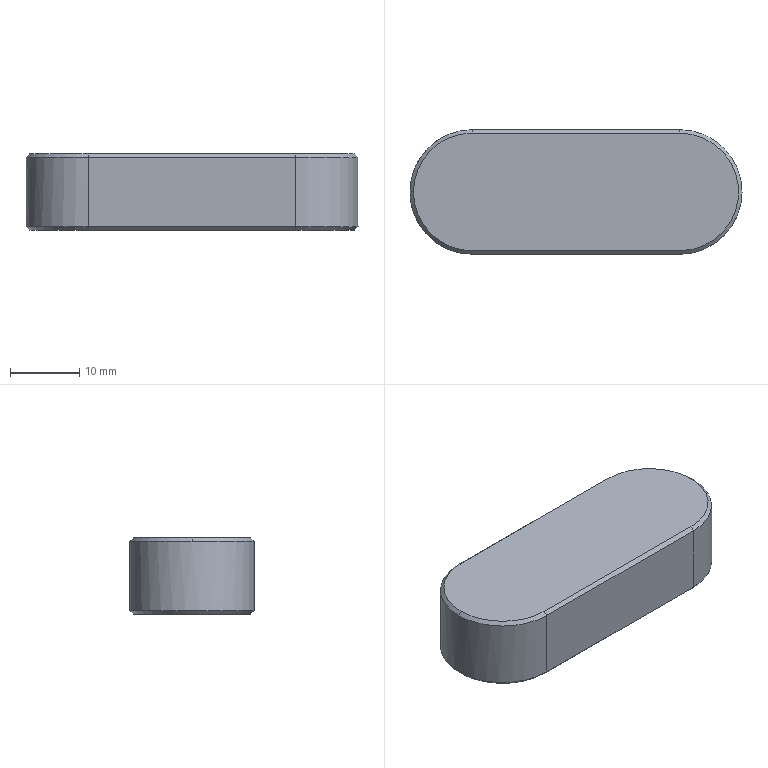Part | SolidWorks | features BaseBody 1 | 1 solid | 17 faces | box 48 x 18 x 11 mm | volume 8710 mm3 | plane 8 | cone 6 | cylinder 3 | commonest cylinder face diameters 18 x3
STEP:
#1=CARTESIAN_POINT('',(-18.723,2.01,11.));
#2=VERTEX_POINT('',#1);
#3=CARTESIAN_POINT('',(-10.223,-6.49,11.));
#4=VERTEX_POINT('',#3);
#5=CARTESIAN_POINT('',(-10.223,2.01,11.));
#6=DIRECTION('',(0.,0.,1.));
#7=DIRECTION('',(-1.,0.,0.));
#8=AXIS2_PLACEMENT_3D('',#5,#6,#7);
#9=CIRCLE('',#8,8.5);
#10=EDGE_CURVE('',#2,#4,#9,.T.);
#11=ORIENTED_EDGE('',*,*,#10,.F.);
#12=CARTESIAN_POINT('',(-19.223,2.01,10.5));
#13=VERTEX_POINT('',#12);
#14=CARTESIAN_POINT('',(-19.223,2.01,10.5));
#15=DIRECTION('',(-0.7071,0.,-0.7071));
#16=VECTOR('',#15,1000.);
#17=LINE('',#14,#16);
#18=EDGE_CURVE('',#2,#13,#17,.T.);
#19=ORIENTED_EDGE('',*,*,#18,.T.);
#20=CARTESIAN_POINT('',(-10.223,-6.99,10.5));
#21=VERTEX_POINT('',#20);
#22=CARTESIAN_POINT('',(-10.223,2.01,10.5));
#23=DIRECTION('',(0.,0.,1.));
#24=DIRECTION('',(0.,1.,0.));
#25=AXIS2_PLACEMENT_3D('',#22,#23,#24);
#26=CIRCLE('',#25,9.);
#27=EDGE_CURVE('',#13,#21,#26,.T.);
#28=ORIENTED_EDGE('',*,*,#27,.T.);
#29=CARTESIAN_POINT('',(-10.223,-6.74,10.75));
#30=DIRECTION('',(0.,0.7071,0.7071));
#31=VECTOR('',#30,1000.);
#32=LINE('',#29,#31);
#33=EDGE_CURVE('',#21,#4,#32,.T.);
#34=ORIENTED_EDGE('',*,*,#33,.T.);
#35=EDGE_LOOP('',(#11,#19,#28,#34));
#36=FACE_OUTER_BOUND('',#35,.T.);
#37=CARTESIAN_POINT('',(-10.223,2.01,10.5));
#38=DIRECTION('',(0.,0.,-1.));
#39=DIRECTION('',(-1.,0.,0.));
#40=AXIS2_PLACEMENT_3D('',#37,#38,#39);
#41=CONICAL_SURFACE('',#40,9.,0.7854);
#42=ADVANCED_FACE('',(#36),#41,.T.);
#43=CARTESIAN_POINT('',(19.777,-6.99,0.5));
#44=VERTEX_POINT('',#43);
#45=CARTESIAN_POINT('',(28.777,2.01,0.5));
#46=VERTEX_POINT('',#45);
#47=CARTESIAN_POINT('',(19.777,2.01,0.5));
#48=DIRECTION('',(0.,0.,1.));
#49=DIRECTION('',(1.,0.,0.));
#50=AXIS2_PLACEMENT_3D('',#47,#48,#49);
#51=CIRCLE('',#50,9.);
#52=EDGE_CURVE('',#44,#46,#51,.T.);
#53=ORIENTED_EDGE('',*,*,#52,.T.);
#54=CARTESIAN_POINT('',(28.777,2.01,10.5));
#55=VERTEX_POINT('',#54);
#56=CARTESIAN_POINT('',(28.777,2.01,0.));
#57=DIRECTION('',(0.,0.,1.));
#58=VECTOR('',#57,1000.);
#59=LINE('',#56,#58);
#60=EDGE_CURVE('',#46,#55,#59,.T.);
#61=ORIENTED_EDGE('',*,*,#60,.T.);
#62=CARTESIAN_POINT('',(19.777,-6.99,10.5));
#63=VERTEX_POINT('',#62);
#64=CARTESIAN_POINT('',(19.777,2.01,10.5));
#65=DIRECTION('',(0.,0.,1.));
#66=DIRECTION('',(0.,-1.,0.));
#67=AXIS2_PLACEMENT_3D('',#64,#65,#66);
#68=CIRCLE('',#67,9.);
#69=EDGE_CURVE('',#63,#55,#68,.T.);
#70=ORIENTED_EDGE('',*,*,#69,.F.);
#71=CARTESIAN_POINT('',(19.777,-6.99,0.));
#72=DIRECTION('',(0.,0.,-1.));
#73=VECTOR('',#72,1000.);
#74=LINE('',#71,#73);
#75=EDGE_CURVE('',#63,#44,#74,.T.);
#76=ORIENTED_EDGE('',*,*,#75,.T.);
#77=EDGE_LOOP('',(#53,#61,#70,#76));
#78=FACE_OUTER_BOUND('',#77,.T.);
#79=CARTESIAN_POINT('',(19.777,2.01,0.));
#80=DIRECTION('',(0.,0.,1.));
#81=DIRECTION('',(1.,0.,0.));
#82=AXIS2_PLACEMENT_3D('',#79,#80,#81);
#83=CYLINDRICAL_SURFACE('',#82,9.);
#84=ADVANCED_FACE('',(#78),#83,.T.);
#85=CARTESIAN_POINT('',(19.777,-6.49,0.));
#86=VERTEX_POINT('',#85);
#87=CARTESIAN_POINT('',(28.277,2.01,0.));
#88=VERTEX_POINT('',#87);
#89=CARTESIAN_POINT('',(19.777,2.01,0.));
#90=DIRECTION('',(0.,0.,1.));
#91=DIRECTION('',(1.,0.,0.));
#92=AXIS2_PLACEMENT_3D('',#89,#90,#91);
#93=CIRCLE('',#92,8.5);
#94=EDGE_CURVE('',#86,#88,#93,.T.);
#95=ORIENTED_EDGE('',*,*,#94,.T.);
#96=CARTESIAN_POINT('',(28.777,2.01,0.5));
#97=DIRECTION('',(0.7071,0.,0.7071));
#98=VECTOR('',#97,1000.);
#99=LINE('',#96,#98);
#100=EDGE_CURVE('',#88,#46,#99,.T.);
#101=ORIENTED_EDGE('',*,*,#100,.T.);
#102=ORIENTED_EDGE('',*,*,#52,.F.);
#103=CARTESIAN_POINT('',(19.777,-6.74,0.25));
#104=DIRECTION('',(0.,0.7071,-0.7071));
#105=VECTOR('',#104,1000.);
#106=LINE('',#103,#105);
#107=EDGE_CURVE('',#44,#86,#106,.T.);
#108=ORIENTED_EDGE('',*,*,#107,.T.);
#109=EDGE_LOOP('',(#95,#101,#102,#108));
#110=FACE_OUTER_BOUND('',#109,.T.);
#111=CARTESIAN_POINT('',(19.777,2.01,0.5));
#112=DIRECTION('',(0.,0.,1.));
#113=DIRECTION('',(1.,0.,0.));
#114=AXIS2_PLACEMENT_3D('',#111,#112,#113);
#115=CONICAL_SURFACE('',#114,9.,0.7854);
#116=ADVANCED_FACE('',(#110),#115,.T.);
#117=CARTESIAN_POINT('',(19.777,10.51,11.));
#118=VERTEX_POINT('',#117);
#119=CARTESIAN_POINT('',(-10.223,10.51,11.));
#120=VERTEX_POINT('',#119);
#121=CARTESIAN_POINT('',(4.777,10.51,11.));
#122=DIRECTION('',(-1.,0.,0.));
#123=VECTOR('',#122,1000.);
#124=LINE('',#121,#123);
#125=EDGE_CURVE('',#118,#120,#124,.T.);
#126=ORIENTED_EDGE('',*,*,#125,.T.);
#127=CARTESIAN_POINT('',(-10.223,2.01,11.));
#128=DIRECTION('',(0.,0.,1.));
#129=DIRECTION('',(-1.,0.,0.));
#130=AXIS2_PLACEMENT_3D('',#127,#128,#129);
#131=CIRCLE('',#130,8.5);
#132=EDGE_CURVE('',#120,#2,#131,.T.);
#133=ORIENTED_EDGE('',*,*,#132,.T.);
#134=ORIENTED_EDGE('',*,*,#10,.T.);
#135=CARTESIAN_POINT('',(19.777,-6.49,11.));
#136=VERTEX_POINT('',#135);
#137=CARTESIAN_POINT('',(4.777,-6.49,11.));
#138=DIRECTION('',(1.,0.,0.));
#139=VECTOR('',#138,1000.);
#140=LINE('',#137,#139);
#141=EDGE_CURVE('',#4,#136,#140,.T.);
#142=ORIENTED_EDGE('',*,*,#141,.T.);
#143=CARTESIAN_POINT('',(19.777,2.01,11.));
#144=DIRECTION('',(0.,0.,1.));
#145=DIRECTION('',(-1.,0.,0.));
#146=AXIS2_PLACEMENT_3D('',#143,#144,#145);
#147=CIRCLE('',#146,8.5);
#148=EDGE_CURVE('',#136,#118,#147,.T.);
#149=ORIENTED_EDGE('',*,*,#148,.T.);
#150=EDGE_LOOP('',(#126,#133,#134,#142,#149));
#151=FACE_OUTER_BOUND('',#150,.T.);
#152=CARTESIAN_POINT('',(4.777,2.01,11.));
#153=DIRECTION('',(0.,0.,1.));
#154=DIRECTION('',(1.,0.,0.));
#155=AXIS2_PLACEMENT_3D('',#152,#153,#154);
#156=PLANE('',#155);
#157=ADVANCED_FACE('',(#151),#156,.T.);
#158=ORIENTED_EDGE('',*,*,#18,.F.);
#159=ORIENTED_EDGE('',*,*,#132,.F.);
#160=CARTESIAN_POINT('',(-10.223,11.01,10.5));
#161=VERTEX_POINT('',#160);
#162=CARTESIAN_POINT('',(-10.223,10.76,10.75));
#163=DIRECTION('',(0.,0.7071,-0.7071));
#164=VECTOR('',#163,1000.);
#165=LINE('',#162,#164);
#166=EDGE_CURVE('',#120,#161,#165,.T.);
#167=ORIENTED_EDGE('',*,*,#166,.T.);
#168=CARTESIAN_POINT('',(-10.223,2.01,10.5));
#169=DIRECTION('',(0.,0.,1.));
#170=DIRECTION('',(0.,1.,0.));
#171=AXIS2_PLACEMENT_3D('',#168,#169,#170);
#172=CIRCLE('',#171,9.);
#173=EDGE_CURVE('',#161,#13,#172,.T.);
#174=ORIENTED_EDGE('',*,*,#173,.T.);
#175=EDGE_LOOP('',(#158,#159,#167,#174));
#176=FACE_OUTER_BOUND('',#175,.T.);
#177=CARTESIAN_POINT('',(-10.223,2.01,10.5));
#178=DIRECTION('',(0.,0.,-1.));
#179=DIRECTION('',(-1.,0.,0.));
#180=AXIS2_PLACEMENT_3D('',#177,#178,#179);
#181=CONICAL_SURFACE('',#180,9.,0.7854);
#182=ADVANCED_FACE('',(#176),#181,.T.);
#183=ORIENTED_EDGE('',*,*,#166,.F.);
#184=ORIENTED_EDGE('',*,*,#125,.F.);
#185=CARTESIAN_POINT('',(19.777,11.01,10.5));
#186=VERTEX_POINT('',#185);
#187=CARTESIAN_POINT('',(19.777,10.76,10.75));
#188=DIRECTION('',(0.,0.7071,-0.7071));
#189=VECTOR('',#188,1000.);
#190=LINE('',#187,#189);
#191=EDGE_CURVE('',#118,#186,#190,.T.);
#192=ORIENTED_EDGE('',*,*,#191,.T.);
#193=CARTESIAN_POINT('',(-2.723,11.01,10.5));
#194=DIRECTION('',(-1.,0.,0.));
#195=VECTOR('',#194,1000.);
#196=LINE('',#193,#195);
#197=EDGE_CURVE('',#186,#161,#196,.T.);
#198=ORIENTED_EDGE('',*,*,#197,.T.);
#199=EDGE_LOOP('',(#183,#184,#192,#198));
#200=FACE_OUTER_BOUND('',#199,.T.);
#201=CARTESIAN_POINT('',(-2.723,10.76,10.75));
#202=DIRECTION('',(0.,0.7071,0.7071));
#203=DIRECTION('',(0.,-0.7071,0.7071));
#204=AXIS2_PLACEMENT_3D('',#201,#202,#203);
#205=PLANE('',#204);
#206=ADVANCED_FACE('',(#200),#205,.T.);
#207=CARTESIAN_POINT('',(19.777,-6.74,10.75));
#208=DIRECTION('',(0.,-0.7071,-0.7071));
#209=VECTOR('',#208,1000.);
#210=LINE('',#207,#209);
#211=EDGE_CURVE('',#136,#63,#210,.T.);
#212=ORIENTED_EDGE('',*,*,#211,.T.);
#213=ORIENTED_EDGE('',*,*,#69,.T.);
#214=CARTESIAN_POINT('',(19.777,2.01,10.5));
#215=DIRECTION('',(0.,0.,1.));
#216=DIRECTION('',(0.,-1.,0.));
#217=AXIS2_PLACEMENT_3D('',#214,#215,#216);
#218=CIRCLE('',#217,9.);
#219=EDGE_CURVE('',#55,#186,#218,.T.);
#220=ORIENTED_EDGE('',*,*,#219,.T.);
#221=ORIENTED_EDGE('',*,*,#191,.F.);
#222=ORIENTED_EDGE('',*,*,#148,.F.);
#223=EDGE_LOOP('',(#212,#213,#220,#221,#222));
#224=FACE_OUTER_BOUND('',#223,.T.);
#225=CARTESIAN_POINT('',(19.777,2.01,10.5));
#226=DIRECTION('',(0.,0.,-1.));
#227=DIRECTION('',(-1.,0.,0.));
#228=AXIS2_PLACEMENT_3D('',#225,#226,#227);
#229=CONICAL_SURFACE('',#228,9.,0.7854);
#230=ADVANCED_FACE('',(#224),#229,.T.);
#231=ORIENTED_EDGE('',*,*,#33,.F.);
#232=CARTESIAN_POINT('',(12.277,-6.99,10.5));
#233=DIRECTION('',(1.,0.,0.));
#234=VECTOR('',#233,1000.);
#235=LINE('',#232,#234);
#236=EDGE_CURVE('',#21,#63,#235,.T.);
#237=ORIENTED_EDGE('',*,*,#236,.T.);
#238=ORIENTED_EDGE('',*,*,#211,.F.);
#239=ORIENTED_EDGE('',*,*,#141,.F.);
#240=EDGE_LOOP('',(#231,#237,#238,#239));
#241=FACE_OUTER_BOUND('',#240,.T.);
#242=CARTESIAN_POINT('',(12.277,-6.74,10.75));
#243=DIRECTION('',(0.,-0.7071,0.7071));
#244=DIRECTION('',(0.,-0.7071,-0.7071));
#245=AXIS2_PLACEMENT_3D('',#242,#243,#244);
#246=PLANE('',#245);
#247=ADVANCED_FACE('',(#241),#246,.T.);
#248=ORIENTED_EDGE('',*,*,#173,.F.);
#249=CARTESIAN_POINT('',(-10.223,11.01,0.5));
#250=VERTEX_POINT('',#249);
#251=CARTESIAN_POINT('',(-10.223,11.01,0.));
#252=DIRECTION('',(0.,0.,-1.));
#253=VECTOR('',#252,1000.);
#254=LINE('',#251,#253);
#255=EDGE_CURVE('',#161,#250,#254,.T.);
#256=ORIENTED_EDGE('',*,*,#255,.T.);
#257=CARTESIAN_POINT('',(-10.223,-6.99,0.5));
#258=VERTEX_POINT('',#257);
#259=CARTESIAN_POINT('',(-10.223,2.01,0.5));
#260=DIRECTION('',(0.,0.,1.));
#261=DIRECTION('',(1.,0.,0.));
#262=AXIS2_PLACEMENT_3D('',#259,#260,#261);
#263=CIRCLE('',#262,9.);
#264=EDGE_CURVE('',#250,#258,#263,.T.);
#265=ORIENTED_EDGE('',*,*,#264,.T.);
#266=CARTESIAN_POINT('',(-10.223,-6.99,0.));
#267=DIRECTION('',(0.,0.,1.));
#268=VECTOR('',#267,1000.);
#269=LINE('',#266,#268);
#270=EDGE_CURVE('',#258,#21,#269,.T.);
#271=ORIENTED_EDGE('',*,*,#270,.T.);
#272=ORIENTED_EDGE('',*,*,#27,.F.);
#273=EDGE_LOOP('',(#248,#256,#265,#271,#272));
#274=FACE_OUTER_BOUND('',#273,.T.);
#275=CARTESIAN_POINT('',(-10.223,2.01,0.));
#276=DIRECTION('',(0.,0.,1.));
#277=DIRECTION('',(1.,0.,0.));
#278=AXIS2_PLACEMENT_3D('',#275,#276,#277);
#279=CYLINDRICAL_SURFACE('',#278,9.);
#280=ADVANCED_FACE('',(#274),#279,.T.);
#281=ORIENTED_EDGE('',*,*,#197,.F.);
#282=CARTESIAN_POINT('',(19.777,11.01,0.5));
#283=VERTEX_POINT('',#282);
#284=CARTESIAN_POINT('',(19.777,11.01,0.));
#285=DIRECTION('',(0.,0.,-1.));
#286=VECTOR('',#285,1000.);
#287=LINE('',#284,#286);
#288=EDGE_CURVE('',#186,#283,#287,.T.);
#289=ORIENTED_EDGE('',*,*,#288,.T.);
#290=CARTESIAN_POINT('',(-10.223,11.01,0.5));
#291=DIRECTION('',(-1.,0.,0.));
#292=VECTOR('',#291,1000.);
#293=LINE('',#290,#292);
#294=EDGE_CURVE('',#283,#250,#293,.T.);
#295=ORIENTED_EDGE('',*,*,#294,.T.);
#296=ORIENTED_EDGE('',*,*,#255,.F.);
#297=EDGE_LOOP('',(#281,#289,#295,#296));
#298=FACE_OUTER_BOUND('',#297,.T.);
#299=CARTESIAN_POINT('',(-10.223,11.01,0.));
#300=DIRECTION('',(0.,1.,0.));
#301=DIRECTION('',(0.,0.,1.));
#302=AXIS2_PLACEMENT_3D('',#299,#300,#301);
#303=PLANE('',#302);
#304=ADVANCED_FACE('',(#298),#303,.T.);
#305=ORIENTED_EDGE('',*,*,#60,.F.);
#306=CARTESIAN_POINT('',(19.777,2.01,0.5));
#307=DIRECTION('',(0.,0.,1.));
#308=DIRECTION('',(1.,0.,0.));
#309=AXIS2_PLACEMENT_3D('',#306,#307,#308);
#310=CIRCLE('',#309,9.);
#311=EDGE_CURVE('',#46,#283,#310,.T.);
#312=ORIENTED_EDGE('',*,*,#311,.T.);
#313=ORIENTED_EDGE('',*,*,#288,.F.);
#314=ORIENTED_EDGE('',*,*,#219,.F.);
#315=EDGE_LOOP('',(#305,#312,#313,#314));
#316=FACE_OUTER_BOUND('',#315,.T.);
#317=CARTESIAN_POINT('',(19.777,2.01,0.));
#318=DIRECTION('',(0.,0.,1.));
#319=DIRECTION('',(1.,0.,0.));
#320=AXIS2_PLACEMENT_3D('',#317,#318,#319);
#321=CYLINDRICAL_SURFACE('',#320,9.);
#322=ADVANCED_FACE('',(#316),#321,.T.);
#323=ORIENTED_EDGE('',*,*,#236,.F.);
#324=ORIENTED_EDGE('',*,*,#270,.F.);
#325=CARTESIAN_POINT('',(19.777,-6.99,0.5));
#326=DIRECTION('',(1.,0.,0.));
#327=VECTOR('',#326,1000.);
#328=LINE('',#325,#327);
#329=EDGE_CURVE('',#258,#44,#328,.T.);
#330=ORIENTED_EDGE('',*,*,#329,.T.);
#331=ORIENTED_EDGE('',*,*,#75,.F.);
#332=EDGE_LOOP('',(#323,#324,#330,#331));
#333=FACE_OUTER_BOUND('',#332,.T.);
#334=CARTESIAN_POINT('',(19.777,-6.99,0.));
#335=DIRECTION('',(0.,-1.,0.));
#336=DIRECTION('',(0.,0.,-1.));
#337=AXIS2_PLACEMENT_3D('',#334,#335,#336);
#338=PLANE('',#337);
#339=ADVANCED_FACE('',(#333),#338,.T.);
#340=CARTESIAN_POINT('',(-10.223,10.51,0.));
#341=VERTEX_POINT('',#340);
#342=CARTESIAN_POINT('',(-10.223,10.76,0.25));
#343=DIRECTION('',(0.,-0.7071,-0.7071));
#344=VECTOR('',#343,1000.);
#345=LINE('',#342,#344);
#346=EDGE_CURVE('',#250,#341,#345,.T.);
#347=ORIENTED_EDGE('',*,*,#346,.T.);
#348=CARTESIAN_POINT('',(-10.223,-6.49,0.));
#349=VERTEX_POINT('',#348);
#350=CARTESIAN_POINT('',(-10.223,2.01,0.));
#351=DIRECTION('',(0.,0.,1.));
#352=DIRECTION('',(1.,0.,0.));
#353=AXIS2_PLACEMENT_3D('',#350,#351,#352);
#354=CIRCLE('',#353,8.5);
#355=EDGE_CURVE('',#341,#349,#354,.T.);
#356=ORIENTED_EDGE('',*,*,#355,.T.);
#357=CARTESIAN_POINT('',(-10.223,-6.74,0.25));
#358=DIRECTION('',(0.,-0.7071,0.7071));
#359=VECTOR('',#358,1000.);
#360=LINE('',#357,#359);
#361=EDGE_CURVE('',#349,#258,#360,.T.);
#362=ORIENTED_EDGE('',*,*,#361,.T.);
#363=ORIENTED_EDGE('',*,*,#264,.F.);
#364=EDGE_LOOP('',(#347,#356,#362,#363));
#365=FACE_OUTER_BOUND('',#364,.T.);
#366=CARTESIAN_POINT('',(-10.223,2.01,0.5));
#367=DIRECTION('',(0.,0.,1.));
#368=DIRECTION('',(1.,0.,0.));
#369=AXIS2_PLACEMENT_3D('',#366,#367,#368);
#370=CONICAL_SURFACE('',#369,9.,0.7854);
#371=ADVANCED_FACE('',(#365),#370,.T.);
#372=CARTESIAN_POINT('',(19.777,10.51,0.));
#373=VERTEX_POINT('',#372);
#374=CARTESIAN_POINT('',(19.777,10.76,0.25));
#375=DIRECTION('',(0.,-0.7071,-0.7071));
#376=VECTOR('',#375,1000.);
#377=LINE('',#374,#376);
#378=EDGE_CURVE('',#283,#373,#377,.T.);
#379=ORIENTED_EDGE('',*,*,#378,.T.);
#380=CARTESIAN_POINT('',(-2.723,10.51,0.));
#381=DIRECTION('',(-1.,0.,0.));
#382=VECTOR('',#381,1000.);
#383=LINE('',#380,#382);
#384=EDGE_CURVE('',#373,#341,#383,.T.);
#385=ORIENTED_EDGE('',*,*,#384,.T.);
#386=ORIENTED_EDGE('',*,*,#346,.F.);
#387=ORIENTED_EDGE('',*,*,#294,.F.);
#388=EDGE_LOOP('',(#379,#385,#386,#387));
#389=FACE_OUTER_BOUND('',#388,.T.);
#390=CARTESIAN_POINT('',(-2.723,10.76,0.25));
#391=DIRECTION('',(0.,0.7071,-0.7071));
#392=DIRECTION('',(0.,0.7071,0.7071));
#393=AXIS2_PLACEMENT_3D('',#390,#391,#392);
#394=PLANE('',#393);
#395=ADVANCED_FACE('',(#389),#394,.T.);
#396=ORIENTED_EDGE('',*,*,#100,.F.);
#397=CARTESIAN_POINT('',(19.777,2.01,0.));
#398=DIRECTION('',(0.,0.,1.));
#399=DIRECTION('',(1.,0.,0.));
#400=AXIS2_PLACEMENT_3D('',#397,#398,#399);
#401=CIRCLE('',#400,8.5);
#402=EDGE_CURVE('',#88,#373,#401,.T.);
#403=ORIENTED_EDGE('',*,*,#402,.T.);
#404=ORIENTED_EDGE('',*,*,#378,.F.);
#405=ORIENTED_EDGE('',*,*,#311,.F.);
#406=EDGE_LOOP('',(#396,#403,#404,#405));
#407=FACE_OUTER_BOUND('',#406,.T.);
#408=CARTESIAN_POINT('',(19.777,2.01,0.5));
#409=DIRECTION('',(0.,0.,1.));
#410=DIRECTION('',(1.,0.,0.));
#411=AXIS2_PLACEMENT_3D('',#408,#409,#410);
#412=CONICAL_SURFACE('',#411,9.,0.7854);
#413=ADVANCED_FACE('',(#407),#412,.T.);
#414=ORIENTED_EDGE('',*,*,#107,.F.);
#415=ORIENTED_EDGE('',*,*,#329,.F.);
#416=ORIENTED_EDGE('',*,*,#361,.F.);
#417=CARTESIAN_POINT('',(12.277,-6.49,0.));
#418=DIRECTION('',(1.,0.,0.));
#419=VECTOR('',#418,1000.);
#420=LINE('',#417,#419);
#421=EDGE_CURVE('',#349,#86,#420,.T.);
#422=ORIENTED_EDGE('',*,*,#421,.T.);
#423=EDGE_LOOP('',(#414,#415,#416,#422));
#424=FACE_OUTER_BOUND('',#423,.T.);
#425=CARTESIAN_POINT('',(12.277,-6.74,0.25));
#426=DIRECTION('',(0.,-0.7071,-0.7071));
#427=DIRECTION('',(0.,0.7071,-0.7071));
#428=AXIS2_PLACEMENT_3D('',#425,#426,#427);
#429=PLANE('',#428);
#430=ADVANCED_FACE('',(#424),#429,.T.);
#431=ORIENTED_EDGE('',*,*,#421,.F.);
#432=ORIENTED_EDGE('',*,*,#355,.F.);
#433=ORIENTED_EDGE('',*,*,#384,.F.);
#434=ORIENTED_EDGE('',*,*,#402,.F.);
#435=ORIENTED_EDGE('',*,*,#94,.F.);
#436=EDGE_LOOP('',(#431,#432,#433,#434,#435));
#437=FACE_OUTER_BOUND('',#436,.T.);
#438=CARTESIAN_POINT('',(4.777,2.01,0.));
#439=DIRECTION('',(0.,0.,1.));
#440=DIRECTION('',(1.,0.,0.));
#441=AXIS2_PLACEMENT_3D('',#438,#439,#440);
#442=PLANE('',#441);
#443=ADVANCED_FACE('',(#437),#442,.F.);
#444=CLOSED_SHELL('',(#42,#84,#116,#157,#182,#206,#230,#247,#280,#304,#322,#339,#371,#395,#413,#430,#443));
#445=MANIFOLD_SOLID_BREP('',#444);
#446=CARTESIAN_POINT('',(0.,0.,0.));
#447=DIRECTION('',(0.,0.,1.));
#448=DIRECTION('',(1.,0.,0.));
#449=AXIS2_PLACEMENT_3D('',#446,#447,#448);
#450=(LENGTH_UNIT()NAMED_UNIT(*)SI_UNIT(.MILLI.,.METRE.));
#451=UNCERTAINTY_MEASURE_WITH_UNIT(LENGTH_MEASURE(0.00001),#450,'','');
#452=(NAMED_UNIT(*)PLANE_ANGLE_UNIT()SI_UNIT($,.RADIAN.));
#453=(NAMED_UNIT(*)SI_UNIT($,.STERADIAN.)SOLID_ANGLE_UNIT());
#454=(GEOMETRIC_REPRESENTATION_CONTEXT(3)GLOBAL_UNCERTAINTY_ASSIGNED_CONTEXT((#451))GLOBAL_UNIT_ASSIGNED_CONTEXT((#450,#452,#453))REPRESENTATION_CONTEXT('',''));
#455=ADVANCED_BREP_SHAPE_REPRESENTATION('',(#445,#449),#454);